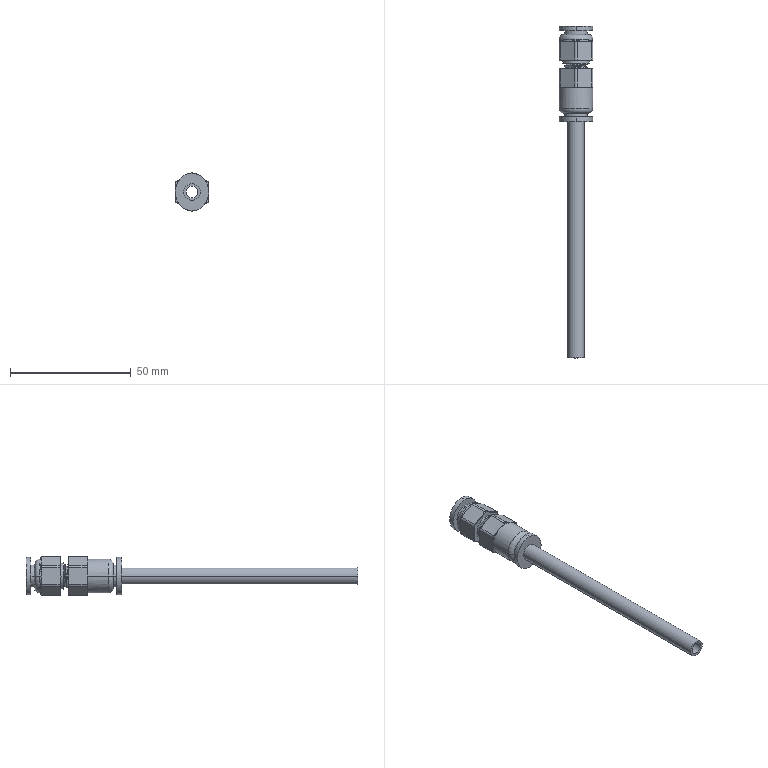Part | SolidWorks | 5 solids | 187 faces | box 14 x 137.38 x 15.856 mm | volume 6154 mm3 | plane 87 | cylinder 82 | spline 8 | torus 6 | cone 4 | commonest cylinder face diameters 2 x12 7.779 x12 9.17 x12 6.9 x10 8.141 x10 9.85 x10